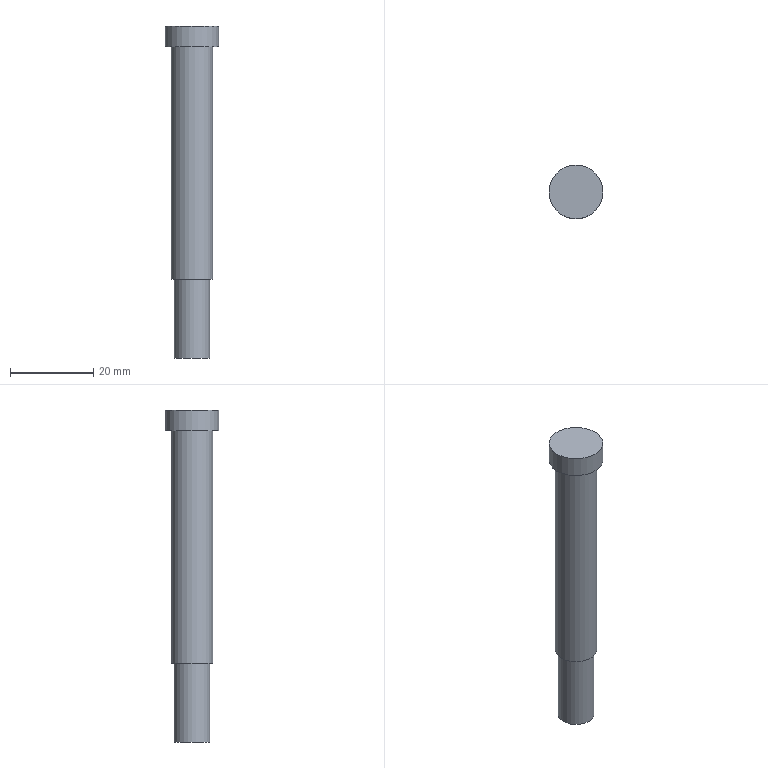Part | NX | features solid 2 | 1 solid | 7 faces | box 13 x 13 x 80 mm | volume 6166 mm3 | plane 4 | cylinder 3 | commonest cylinder face diameters 8.6 x1 10 x1 13 x1
STEP:
#1=CARTESIAN_POINT('',(-640.553,-254.178,59.));
#2=VERTEX_POINT('',#1);
#3=CARTESIAN_POINT('',(-645.553,-254.178,59.));
#4=DIRECTION('',(0.,0.,1.));
#5=DIRECTION('',(1.,0.,0.));
#6=AXIS2_PLACEMENT_3D('',#3,#4,#5);
#7=CIRCLE('',#6,5.);
#8=EDGE_CURVE('',#2,#2,#7,.T.);
#9=ORIENTED_EDGE('',*,*,#8,.T.);
#10=EDGE_LOOP('',(#9));
#11=FACE_BOUND('',#10,.T.);
#12=CARTESIAN_POINT('',(-640.553,-254.178,115.));
#13=VERTEX_POINT('',#12);
#14=CARTESIAN_POINT('',(-645.553,-254.178,115.));
#15=DIRECTION('',(0.,0.,1.));
#16=DIRECTION('',(1.,0.,0.));
#17=AXIS2_PLACEMENT_3D('',#14,#15,#16);
#18=CIRCLE('',#17,5.);
#19=EDGE_CURVE('',#13,#13,#18,.T.);
#20=ORIENTED_EDGE('',*,*,#19,.F.);
#21=EDGE_LOOP('',(#20));
#22=FACE_BOUND('',#21,.T.);
#23=CARTESIAN_POINT('',(-645.553,-254.178,120.));
#24=DIRECTION('',(0.,0.,-1.));
#25=DIRECTION('',(-1.,0.,0.));
#26=AXIS2_PLACEMENT_3D('',#23,#24,#25);
#27=CYLINDRICAL_SURFACE('',#26,5.);
#28=ADVANCED_FACE('',(#11,#22),#27,.T.);
#29=CARTESIAN_POINT('',(-641.253,-254.178,59.));
#30=VERTEX_POINT('',#29);
#31=CARTESIAN_POINT('',(-645.553,-254.178,59.));
#32=DIRECTION('',(0.,0.,1.));
#33=DIRECTION('',(1.,0.,0.));
#34=AXIS2_PLACEMENT_3D('',#31,#32,#33);
#35=CIRCLE('',#34,4.3);
#36=EDGE_CURVE('',#30,#30,#35,.T.);
#37=ORIENTED_EDGE('',*,*,#36,.T.);
#38=EDGE_LOOP('',(#37));
#39=FACE_BOUND('',#38,.T.);
#40=ORIENTED_EDGE('',*,*,#8,.F.);
#41=EDGE_LOOP('',(#40));
#42=FACE_BOUND('',#41,.T.);
#43=CARTESIAN_POINT('',(-645.553,-254.178,59.));
#44=DIRECTION('',(0.,0.,1.));
#45=DIRECTION('',(1.,0.,0.));
#46=AXIS2_PLACEMENT_3D('',#43,#44,#45);
#47=PLANE('',#46);
#48=ADVANCED_FACE('',(#39,#42),#47,.F.);
#49=CARTESIAN_POINT('',(-639.053,-254.178,115.));
#50=VERTEX_POINT('',#49);
#51=CARTESIAN_POINT('',(-645.553,-254.178,115.));
#52=DIRECTION('',(0.,0.,1.));
#53=DIRECTION('',(1.,0.,0.));
#54=AXIS2_PLACEMENT_3D('',#51,#52,#53);
#55=CIRCLE('',#54,6.5);
#56=EDGE_CURVE('',#50,#50,#55,.T.);
#57=ORIENTED_EDGE('',*,*,#56,.F.);
#58=EDGE_LOOP('',(#57));
#59=FACE_BOUND('',#58,.T.);
#60=ORIENTED_EDGE('',*,*,#19,.T.);
#61=EDGE_LOOP('',(#60));
#62=FACE_BOUND('',#61,.T.);
#63=CARTESIAN_POINT('',(-645.553,-254.178,115.));
#64=DIRECTION('',(0.,0.,1.));
#65=DIRECTION('',(1.,0.,0.));
#66=AXIS2_PLACEMENT_3D('',#63,#64,#65);
#67=PLANE('',#66);
#68=ADVANCED_FACE('',(#59,#62),#67,.F.);
#69=ORIENTED_EDGE('',*,*,#56,.T.);
#70=EDGE_LOOP('',(#69));
#71=FACE_BOUND('',#70,.T.);
#72=CARTESIAN_POINT('',(-639.053,-254.178,120.));
#73=VERTEX_POINT('',#72);
#74=CARTESIAN_POINT('',(-645.553,-254.178,120.));
#75=DIRECTION('',(0.,0.,1.));
#76=DIRECTION('',(1.,0.,0.));
#77=AXIS2_PLACEMENT_3D('',#74,#75,#76);
#78=CIRCLE('',#77,6.5);
#79=EDGE_CURVE('',#73,#73,#78,.T.);
#80=ORIENTED_EDGE('',*,*,#79,.F.);
#81=EDGE_LOOP('',(#80));
#82=FACE_BOUND('',#81,.T.);
#83=CARTESIAN_POINT('',(-645.553,-254.178,115.));
#84=DIRECTION('',(0.,0.,1.));
#85=DIRECTION('',(1.,0.,0.));
#86=AXIS2_PLACEMENT_3D('',#83,#84,#85);
#87=CYLINDRICAL_SURFACE('',#86,6.5);
#88=ADVANCED_FACE('',(#71,#82),#87,.T.);
#89=ORIENTED_EDGE('',*,*,#79,.T.);
#90=EDGE_LOOP('',(#89));
#91=FACE_BOUND('',#90,.T.);
#92=CARTESIAN_POINT('',(-645.553,-254.178,120.));
#93=DIRECTION('',(0.,0.,1.));
#94=DIRECTION('',(1.,0.,0.));
#95=AXIS2_PLACEMENT_3D('',#92,#93,#94);
#96=PLANE('',#95);
#97=ADVANCED_FACE('',(#91),#96,.T.);
#98=CARTESIAN_POINT('',(-641.253,-254.178,40.));
#99=VERTEX_POINT('',#98);
#100=CARTESIAN_POINT('',(-645.553,-254.178,40.));
#101=DIRECTION('',(0.,0.,1.));
#102=DIRECTION('',(1.,0.,0.));
#103=AXIS2_PLACEMENT_3D('',#100,#101,#102);
#104=CIRCLE('',#103,4.3);
#105=EDGE_CURVE('',#99,#99,#104,.T.);
#106=ORIENTED_EDGE('',*,*,#105,.T.);
#107=EDGE_LOOP('',(#106));
#108=FACE_BOUND('',#107,.T.);
#109=ORIENTED_EDGE('',*,*,#36,.F.);
#110=EDGE_LOOP('',(#109));
#111=FACE_BOUND('',#110,.T.);
#112=CARTESIAN_POINT('',(-645.553,-254.178,40.));
#113=DIRECTION('',(0.,0.,1.));
#114=DIRECTION('',(1.,0.,0.));
#115=AXIS2_PLACEMENT_3D('',#112,#113,#114);
#116=CYLINDRICAL_SURFACE('',#115,4.3);
#117=ADVANCED_FACE('',(#108,#111),#116,.T.);
#118=ORIENTED_EDGE('',*,*,#105,.F.);
#119=EDGE_LOOP('',(#118));
#120=FACE_BOUND('',#119,.T.);
#121=CARTESIAN_POINT('',(-645.553,-254.178,40.));
#122=DIRECTION('',(0.,0.,1.));
#123=DIRECTION('',(1.,0.,0.));
#124=AXIS2_PLACEMENT_3D('',#121,#122,#123);
#125=PLANE('',#124);
#126=ADVANCED_FACE('',(#120),#125,.F.);
#127=CLOSED_SHELL('',(#28,#48,#68,#88,#97,#117,#126));
#128=MANIFOLD_SOLID_BREP('',#127);
#129=(LENGTH_UNIT()NAMED_UNIT(*)SI_UNIT(.MILLI.,.METRE.));
#130=UNCERTAINTY_MEASURE_WITH_UNIT(LENGTH_MEASURE(0.00001),#129,'','');
#131=(NAMED_UNIT(*)PLANE_ANGLE_UNIT()SI_UNIT($,.RADIAN.));
#132=(NAMED_UNIT(*)SI_UNIT($,.STERADIAN.)SOLID_ANGLE_UNIT());
#133=(GEOMETRIC_REPRESENTATION_CONTEXT(3)GLOBAL_UNCERTAINTY_ASSIGNED_CONTEXT((#130))GLOBAL_UNIT_ASSIGNED_CONTEXT((#129,#131,#132))REPRESENTATION_CONTEXT('',''));
#134=ADVANCED_BREP_SHAPE_REPRESENTATION('',(#128),#133);